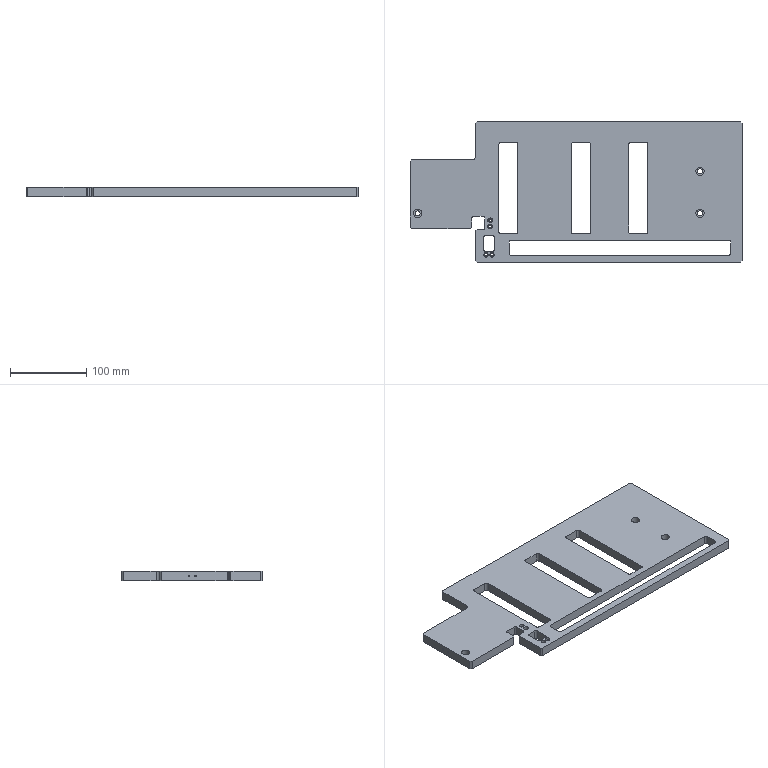NC program | NX | posted with a generic post | part box 435 x 184 x 12 mm
Lines 10012 to 10210 of 10210:
(PLANAR_MILL_COPY_COPY_COPY_COPY_COPY_COPY_1_COPY_COPY , TOOL : D6A45)
N19944 T01 M6
N19946 G54
N19948 G17 G0 G90 X166.6 Y-28.866 S9500 M3
N19950 G43 Z30. H1
N19952 Z0.5
N19954 G94 G1 Z-1. F1250.
N19956 G3 X167.1 Y-28. R1.
N19958 X162.5 Y-23.4 R4.6
N19960 X167.1 Y-28. R-4.6
N19962 X166.6 Y-27.134 R1.
N19964 G1 Z0.5
N19966 G0 Z30.
N19968 Y26.134
N19970 Z0.5
N19972 G1 Z-1.
N19974 G3 X167.1 Y27. R1.
N19976 X162.5 Y31.6 R4.6
N19978 X167.1 Y27. R-4.6
N19980 X166.6 Y27.866 R1.
N19982 G1 Z0.5
N19984 G0 Z30.
N19986 X92.6 Y4.134
N19988 Z0.5
N19990 G1 Z-1.
N19992 G3 X93.1 Y5. R1.
N19994 G1 Y62.5
N19996 G3 X91.5 Y64.1 R1.6
N19998 G1 X71.5
N20000 G3 X69.9 Y62.5 R1.6
N20002 G1 Y-52.5
N20004 G3 X71.5 Y-54.1 R1.6
N20006 G1 X91.5
N20008 G3 X93.1 Y-52.5 R1.6
N20010 G1 Y5.
N20012 G3 X92.6 Y5.866 R1.
N20014 G1 Z0.5
N20016 G0 Z30.
N20018 X56.634 Y-81.6
N20020 Z0.5
N20022 G1 Z-1.
N20024 G3 X57.5 Y-82.1 R1.
N20026 G1 X200.
N20028 G3 X201.6 Y-80.5 R1.6
N20030 G1 Y-65.5
N20032 G3 X200. Y-63.9 R1.6
N20034 G1 X-85.
N20036 G3 X-86.6 Y-65.5 R1.6
N20038 G1 Y-80.5
N20040 G3 X-85. Y-82.1 R1.6
N20042 G1 X57.5
N20044 G3 X58.366 Y-81.6 R1.
N20046 G1 Z0.5
N20048 G0 Z30.
N20050 X43.866 Y-93.4
N20052 Z0.5
N20054 G1 Z-1.
N20056 G3 X43. Y-92.9 R1.
N20058 G1 X-129.5
N20060 G2 X-130.136 Y-92.636 R0.9
N20062 G1 X-132.136 Y-90.636
N20064 G2 X-132.4 Y-90. R0.9
N20066 G1 Y-51.
N20068 G2 X-132.136 Y-50.364 R0.9
N20070 G1 X-130.136 Y-48.364
N20072 G2 X-129.5 Y-48.1 R0.9
N20074 G1 X-121.5
N20076 G3 X-120.4 Y-47. R1.1
N20078 G1 Y-34.
N20080 G3 X-121.5 Y-32.9 R1.1
N20082 G1 X-134.5
N20084 G3 X-135.6 Y-34. R1.1
N20086 G1 Y-46.
N20088 G2 X-135.864 Y-46.636 R0.9
N20090 G1 X-137.864 Y-48.636
N20092 G2 X-138.5 Y-48.9 R0.9
N20094 G1 X-215.5
N20096 G2 X-216.136 Y-48.636 R0.9
N20098 G1 X-218.136 Y-46.636
N20100 G2 X-218.4 Y-46. R0.9
N20102 G1 Y40.
N20104 G2 X-218.136 Y40.636 R0.9
N20106 G1 X-216.136 Y42.636
N20108 G2 X-215.5 Y42.9 R0.9
N20110 G1 X-136.5
N20112 G3 X-132.4 Y47. R4.1
N20114 G1 Y90.
N20116 G2 X-132.136 Y90.636 R0.9
N20118 G1 X-130.136 Y92.636
N20120 G2 X-129.5 Y92.9 R0.9
N20122 G1 X215.5
N20124 G2 X216.136 Y92.636 R0.9
N20126 G1 X218.136 Y90.636
N20128 G2 X218.4 Y90. R0.9
N20130 G1 Y-90.
N20132 G2 X218.136 Y-90.636 R0.9
N20134 G1 X216.136 Y-92.636
N20136 G2 X215.5 Y-92.9 R0.9
N20138 G1 X43.
N20140 G3 X42.134 Y-93.4 R1.
N20142 G1 Z0.5
N20144 G0 Z30.
N20146 X17.6 Y4.134
N20148 Z0.5
N20150 G1 Z-1.
N20152 G3 X18.1 Y5. R1.
N20154 G1 Y62.5
N20156 G3 X16.5 Y64.1 R1.6
N20158 G1 X-3.5
N20160 G3 X-5.1 Y62.5 R1.6
N20162 G1 Y-52.5
N20164 G3 X-3.5 Y-54.1 R1.6
N20166 G1 X16.5
N20168 G3 X18.1 Y-52.5 R1.6
N20170 G1 Y5.
N20172 G3 X17.6 Y5.866 R1.
N20174 G1 Z0.5
N20176 G0 Z30.
N20178 X-77.4 Y4.134
N20180 Z0.5
N20182 G1 Z-1.
N20184 G3 X-76.9 Y5. R1.
N20186 G1 Y62.
N20188 G3 X-79. Y64.1 R2.1
N20190 G1 X-98.
N20192 G3 X-100.1 Y62. R2.1
N20194 G1 Y-52.
N20196 G3 X-98. Y-54.1 R2.1
N20198 G1 X-79.
N20200 G3 X-76.9 Y-52. R2.1
N20202 G1 Y5.
N20204 G3 X-77.4 Y5.866 R1.
N20206 G1 Z0.5
N20208 G0 Z30.
N20210 X-113.366 Y-38.6
N20212 Z0.5
N20214 G1 Z-1.
N20216 G3 X-112.5 Y-39.1 R1.
N20218 X-110.4 Y-37. R2.1
N20220 X-112.5 Y-39.1 R-2.1
N20222 X-111.634 Y-38.6 R1.
N20224 G1 Z0.5
N20226 G0 Z30.
N20228 X-113.366 Y-46.6
N20230 Z0.5
N20232 G1 Z-1.
N20234 G3 X-112.5 Y-47.1 R1.
N20236 X-110.4 Y-45. R2.1
N20238 X-112.5 Y-47.1 R-2.1
N20240 X-111.634 Y-46.6 R1.
N20242 G1 Z0.5
N20244 G0 Z30.
N20246 X-107.9 Y-68.366
N20248 Z0.5
N20250 G1 Z-1.
N20252 G3 X-107.4 Y-67.5 R1.
N20254 G1 Y-60.
N20256 G3 X-109. Y-58.4 R1.6
N20258 G1 X-119.
N20260 G3 X-120.6 Y-60. R1.6
N20262 G1 Y-75.
N20264 G3 X-119. Y-76.6 R1.6
N20266 G1 X-109.
N20268 G3 X-107.4 Y-75. R1.6
N20270 G1 Y-67.5
N20272 G3 X-107.9 Y-66.634 R1.
N20274 G1 Z0.5
N20276 G0 Z30.
N20278 X-110.866 Y-84.1
N20280 Z0.5
N20282 G1 Z-1.
N20284 G3 X-110. Y-84.6 R1.
N20286 X-107.9 Y-82.5 R2.1
N20288 X-110. Y-84.6 R-2.1
N20290 X-109.134 Y-84.1 R1.
N20292 G1 Z0.5
N20294 G0 Z30.
N20296 X-118.866
N20298 Z0.5
N20300 G1 Z-1.
N20302 G3 X-118. Y-84.6 R1.
N20304 X-115.9 Y-82.5 R2.1
N20306 X-118. Y-84.6 R-2.1
N20308 X-117.134 Y-84.1 R1.
N20310 G1 Z0.5
N20312 G0 Z30.
N20314 X-211.6 Y-27.134
N20316 Z0.5
N20318 G1 Z-1.
N20320 G3 X-212.1 Y-28. R1.
N20322 X-207.5 Y-32.6 R4.6
N20324 X-212.1 Y-28. R-4.6
N20326 X-211.6 Y-28.866 R1.
N20328 G1 Z0.5
N20330 G0 Z30.
N20332 M5
N20334 M2